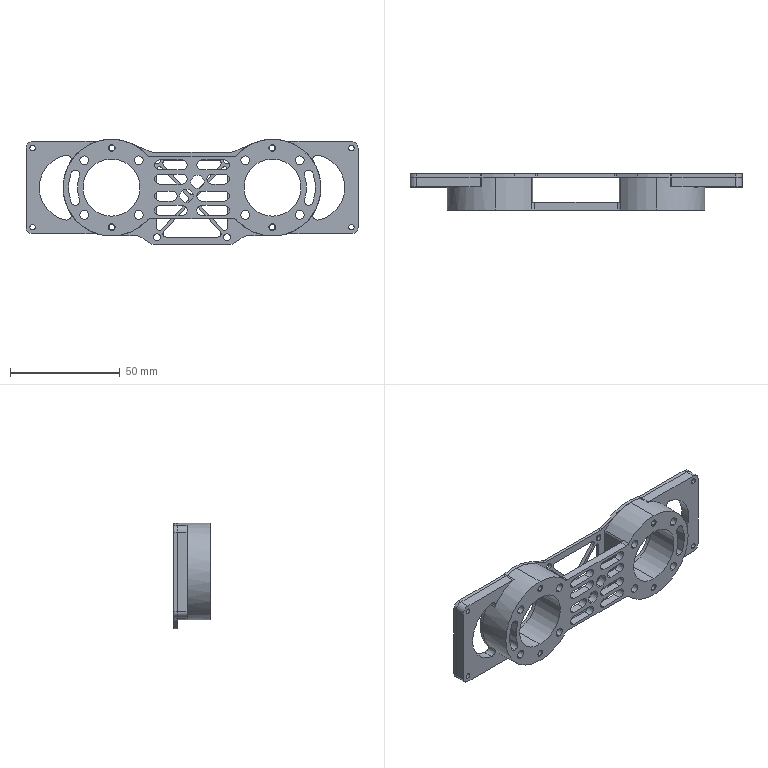Part | SolidWorks | features ICE 7, Fillet 6, Extrusion 1, HoleWzd 1 | 2 solids | 307 faces | box 151 x 16.5 x 48 mm | volume 33794 mm3 | cylinder 225 | plane 74 | cone 8 | commonest cylinder face diameters 3 x39 6 x30 4 x22 2.5 x16 3.15 x16 4.02 x16